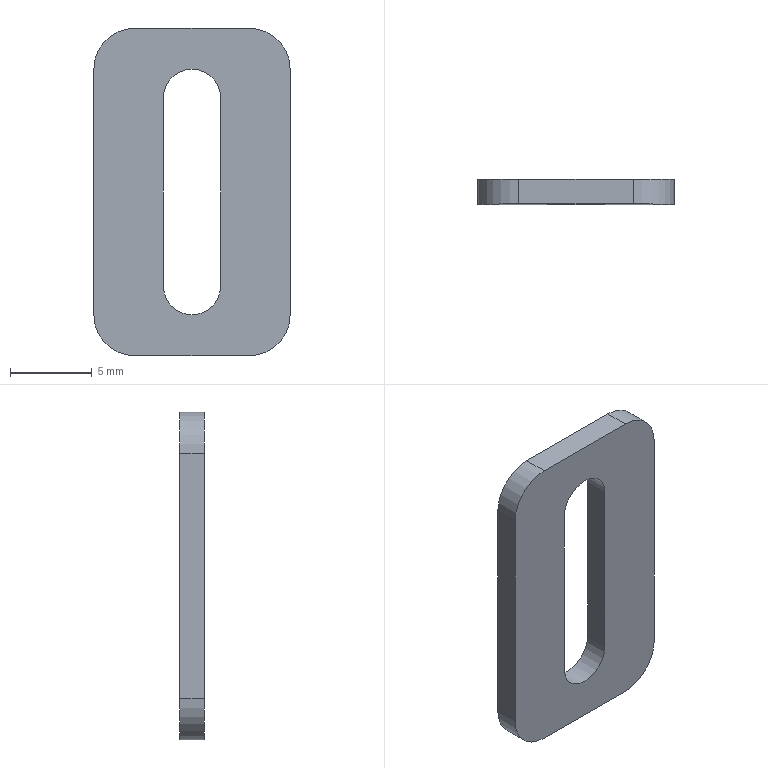Part | STEP file | Glass fixing block 001 | 1 solid | 15 faces | box 12 x 1.5 x 20 mm | volume 277.146 mm3 | plane 8 | cylinder 7 | commonest cylinder face diameters 5 x4 3.5 x3
STEP:
#1=CARTESIAN_POINT('',(0.,0.,0.));
#2=DIRECTION('',(0.,0.,1.));
#3=DIRECTION('',(1.,0.,0.));
#4=AXIS2_PLACEMENT_3D('',#1,#2,#3);
#5=CARTESIAN_POINT('',(1.75,0.,5.75));
#6=VERTEX_POINT('',#5);
#7=CARTESIAN_POINT('',(1.75,1.5,5.75));
#8=VERTEX_POINT('',#7);
#9=CARTESIAN_POINT('',(1.75,0.,5.75));
#10=DIRECTION('',(0.,1.,0.));
#11=VECTOR('',#10,1.);
#12=LINE('',#9,#11);
#13=CARTESIAN_POINT('',(0.,0.,5.75));
#14=DIRECTION('',(0.,1.,0.));
#15=DIRECTION('',(0.,0.,1.));
#16=AXIS2_PLACEMENT_3D('',#13,#14,#15);
#17=CYLINDRICAL_SURFACE('',#16,1.75);
#18=CARTESIAN_POINT('',(1.571,0.));
#19=DIRECTION('',(0.,1.));
#20=VECTOR('',#19,1.);
#21=LINE('',#18,#20);
#22=(GEOMETRIC_REPRESENTATION_CONTEXT(2)PARAMETRIC_REPRESENTATION_CONTEXT()REPRESENTATION_CONTEXT('',''));
#23=DEFINITIONAL_REPRESENTATION('',(#21),#22);
#24=PCURVE('',#17,#23);
#25=CARTESIAN_POINT('',(1.75,0.,5.75));
#26=DIRECTION('',(1.,0.,0.));
#27=DIRECTION('',(0.,0.,-1.));
#28=AXIS2_PLACEMENT_3D('',#25,#26,#27);
#29=PLANE('',#28);
#30=CARTESIAN_POINT('',(0.,0.));
#31=DIRECTION('',(0.,1.));
#32=VECTOR('',#31,1.);
#33=LINE('',#30,#32);
#34=(GEOMETRIC_REPRESENTATION_CONTEXT(2)PARAMETRIC_REPRESENTATION_CONTEXT()REPRESENTATION_CONTEXT('',''));
#35=DEFINITIONAL_REPRESENTATION('',(#33),#34);
#36=PCURVE('',#29,#35);
#37=SURFACE_CURVE('',#12,(#24,#36),.PCURVE_S1.);
#38=EDGE_CURVE('',#6,#8,#37,.T.);
#39=ORIENTED_EDGE('',*,*,#38,.T.);
#40=CARTESIAN_POINT('',(0.,1.5,7.5));
#41=VERTEX_POINT('',#40);
#42=CARTESIAN_POINT('',(0.,1.5,5.75));
#43=DIRECTION('',(0.,1.,0.));
#44=DIRECTION('',(0.,0.,1.));
#45=AXIS2_PLACEMENT_3D('',#42,#43,#44);
#46=CIRCLE('',#45,1.75);
#47=CARTESIAN_POINT('',(0.,1.5));
#48=DIRECTION('',(1.,0.));
#49=VECTOR('',#48,1.);
#50=LINE('',#47,#49);
#51=(GEOMETRIC_REPRESENTATION_CONTEXT(2)PARAMETRIC_REPRESENTATION_CONTEXT()REPRESENTATION_CONTEXT('',''));
#52=DEFINITIONAL_REPRESENTATION('',(#50),#51);
#53=PCURVE('',#17,#52);
#54=CARTESIAN_POINT('',(0.,1.5,0.));
#55=DIRECTION('',(0.,-1.,0.));
#56=DIRECTION('',(0.,0.,-1.));
#57=AXIS2_PLACEMENT_3D('',#54,#55,#56);
#58=PLANE('',#57);
#59=CARTESIAN_POINT('',(-7.5,0.));
#60=CARTESIAN_POINT('',(-7.5,3.031));
#61=CARTESIAN_POINT('',(-4.875,1.516));
#62=CARTESIAN_POINT('',(-2.25,0.));
#63=CARTESIAN_POINT('',(-4.875,-1.516));
#64=CARTESIAN_POINT('',(-7.5,-3.031));
#65=CARTESIAN_POINT('',(-7.5,0.));
#66=(BOUNDED_CURVE()B_SPLINE_CURVE(2,(#59,#60,#61,#62,#63,#64,#65),.UNSPECIFIED.,.T.,.F.)B_SPLINE_CURVE_WITH_KNOTS((1,2,2,2,2,1),(-2.094,0.,2.094,4.189,6.283,8.378),.UNSPECIFIED.)CURVE()GEOMETRIC_REPRESENTATION_ITEM()RATIONAL_B_SPLINE_CURVE((1.,0.5,1.,0.5,1.,0.5,1.))REPRESENTATION_ITEM(''));
#67=(GEOMETRIC_REPRESENTATION_CONTEXT(2)PARAMETRIC_REPRESENTATION_CONTEXT()REPRESENTATION_CONTEXT('',''));
#68=DEFINITIONAL_REPRESENTATION('',(#66),#67);
#69=PCURVE('',#58,#68);
#70=SURFACE_CURVE('',#46,(#53,#69),.PCURVE_S1.);
#71=EDGE_CURVE('',#41,#8,#70,.T.);
#72=ORIENTED_EDGE('',*,*,#71,.F.);
#73=CARTESIAN_POINT('',(0.,0.,7.5));
#74=VERTEX_POINT('',#73);
#75=CARTESIAN_POINT('',(0.,0.,7.5));
#76=DIRECTION('',(0.,1.,0.));
#77=VECTOR('',#76,1.);
#78=LINE('',#75,#77);
#79=CARTESIAN_POINT('',(0.,0.));
#80=DIRECTION('',(0.,1.));
#81=VECTOR('',#80,1.);
#82=LINE('',#79,#81);
#83=(GEOMETRIC_REPRESENTATION_CONTEXT(2)PARAMETRIC_REPRESENTATION_CONTEXT()REPRESENTATION_CONTEXT('',''));
#84=DEFINITIONAL_REPRESENTATION('',(#82),#83);
#85=PCURVE('',#17,#84);
#86=CARTESIAN_POINT('',(0.,0.,5.75));
#87=DIRECTION('',(0.,1.,0.));
#88=DIRECTION('',(0.,0.,1.));
#89=AXIS2_PLACEMENT_3D('',#86,#87,#88);
#90=CYLINDRICAL_SURFACE('',#89,1.75);
#91=CARTESIAN_POINT('',(6.283,0.));
#92=DIRECTION('',(0.,1.));
#93=VECTOR('',#92,1.);
#94=LINE('',#91,#93);
#95=(GEOMETRIC_REPRESENTATION_CONTEXT(2)PARAMETRIC_REPRESENTATION_CONTEXT()REPRESENTATION_CONTEXT('',''));
#96=DEFINITIONAL_REPRESENTATION('',(#94),#95);
#97=PCURVE('',#90,#96);
#98=SURFACE_CURVE('',#78,(#85,#97),.PCURVE_S1.);
#99=EDGE_CURVE('',#74,#41,#98,.T.);
#100=ORIENTED_EDGE('',*,*,#99,.F.);
#101=CARTESIAN_POINT('',(0.,0.,5.75));
#102=DIRECTION('',(0.,1.,0.));
#103=DIRECTION('',(0.,0.,1.));
#104=AXIS2_PLACEMENT_3D('',#101,#102,#103);
#105=CIRCLE('',#104,1.75);
#106=CARTESIAN_POINT('',(0.,0.));
#107=DIRECTION('',(1.,0.));
#108=VECTOR('',#107,1.);
#109=LINE('',#106,#108);
#110=(GEOMETRIC_REPRESENTATION_CONTEXT(2)PARAMETRIC_REPRESENTATION_CONTEXT()REPRESENTATION_CONTEXT('',''));
#111=DEFINITIONAL_REPRESENTATION('',(#109),#110);
#112=PCURVE('',#17,#111);
#113=CARTESIAN_POINT('',(0.,0.,0.));
#114=DIRECTION('',(0.,-1.,0.));
#115=DIRECTION('',(0.,0.,-1.));
#116=AXIS2_PLACEMENT_3D('',#113,#114,#115);
#117=PLANE('',#116);
#118=CARTESIAN_POINT('',(-7.5,0.));
#119=CARTESIAN_POINT('',(-7.5,3.031));
#120=CARTESIAN_POINT('',(-4.875,1.516));
#121=CARTESIAN_POINT('',(-2.25,0.));
#122=CARTESIAN_POINT('',(-4.875,-1.516));
#123=CARTESIAN_POINT('',(-7.5,-3.031));
#124=CARTESIAN_POINT('',(-7.5,0.));
#125=(BOUNDED_CURVE()B_SPLINE_CURVE(2,(#118,#119,#120,#121,#122,#123,#124),.UNSPECIFIED.,.T.,.F.)B_SPLINE_CURVE_WITH_KNOTS((1,2,2,2,2,1),(-2.094,0.,2.094,4.189,6.283,8.378),.UNSPECIFIED.)CURVE()GEOMETRIC_REPRESENTATION_ITEM()RATIONAL_B_SPLINE_CURVE((1.,0.5,1.,0.5,1.,0.5,1.))REPRESENTATION_ITEM(''));
#126=(GEOMETRIC_REPRESENTATION_CONTEXT(2)PARAMETRIC_REPRESENTATION_CONTEXT()REPRESENTATION_CONTEXT('',''));
#127=DEFINITIONAL_REPRESENTATION('',(#125),#126);
#128=PCURVE('',#117,#127);
#129=SURFACE_CURVE('',#105,(#112,#128),.PCURVE_S1.);
#130=EDGE_CURVE('',#74,#6,#129,.T.);
#131=ORIENTED_EDGE('',*,*,#130,.T.);
#132=EDGE_LOOP('',(#39,#72,#100,#131));
#133=FACE_BOUND('',#132,.F.);
#134=ADVANCED_FACE('',(#133),#17,.F.);
#135=CARTESIAN_POINT('',(6.,0.,7.5));
#136=VERTEX_POINT('',#135);
#137=CARTESIAN_POINT('',(6.,0.,-7.5));
#138=VERTEX_POINT('',#137);
#139=CARTESIAN_POINT('',(6.,0.,10.));
#140=DIRECTION('',(0.,0.,-1.));
#141=VECTOR('',#140,1.);
#142=LINE('',#139,#141);
#143=CARTESIAN_POINT('',(6.,1.5,10.));
#144=DIRECTION('',(-1.,0.,0.));
#145=DIRECTION('',(0.,0.,1.));
#146=AXIS2_PLACEMENT_3D('',#143,#144,#145);
#147=PLANE('',#146);
#148=CARTESIAN_POINT('',(0.,-1.5));
#149=DIRECTION('',(-1.,0.));
#150=VECTOR('',#149,1.);
#151=LINE('',#148,#150);
#152=(GEOMETRIC_REPRESENTATION_CONTEXT(2)PARAMETRIC_REPRESENTATION_CONTEXT()REPRESENTATION_CONTEXT('',''));
#153=DEFINITIONAL_REPRESENTATION('',(#151),#152);
#154=PCURVE('',#147,#153);
#155=CARTESIAN_POINT('',(-10.,6.));
#156=DIRECTION('',(1.,0.));
#157=VECTOR('',#156,1.);
#158=LINE('',#155,#157);
#159=(GEOMETRIC_REPRESENTATION_CONTEXT(2)PARAMETRIC_REPRESENTATION_CONTEXT()REPRESENTATION_CONTEXT('',''));
#160=DEFINITIONAL_REPRESENTATION('',(#158),#159);
#161=PCURVE('',#117,#160);
#162=SURFACE_CURVE('',#142,(#154,#161),.PCURVE_S1.);
#163=EDGE_CURVE('',#136,#138,#162,.T.);
#164=ORIENTED_EDGE('',*,*,#163,.T.);
#165=CARTESIAN_POINT('',(6.,1.5,-7.5));
#166=VERTEX_POINT('',#165);
#167=CARTESIAN_POINT('',(6.,1.5,-7.5));
#168=DIRECTION('',(0.,1.,0.));
#169=VECTOR('',#168,1.);
#170=LINE('',#167,#169);
#171=CARTESIAN_POINT('',(-17.5,0.));
#172=DIRECTION('',(0.,1.));
#173=VECTOR('',#172,1.);
#174=LINE('',#171,#173);
#175=(GEOMETRIC_REPRESENTATION_CONTEXT(2)PARAMETRIC_REPRESENTATION_CONTEXT()REPRESENTATION_CONTEXT('',''));
#176=DEFINITIONAL_REPRESENTATION('',(#174),#175);
#177=PCURVE('',#147,#176);
#178=CARTESIAN_POINT('',(3.5,1.5,-7.5));
#179=DIRECTION('',(0.,-1.,0.));
#180=DIRECTION('',(0.,0.,-1.));
#181=AXIS2_PLACEMENT_3D('',#178,#179,#180);
#182=CYLINDRICAL_SURFACE('',#181,2.5);
#183=CARTESIAN_POINT('',(1.571,0.));
#184=DIRECTION('',(0.,-1.));
#185=VECTOR('',#184,1.);
#186=LINE('',#183,#185);
#187=(GEOMETRIC_REPRESENTATION_CONTEXT(2)PARAMETRIC_REPRESENTATION_CONTEXT()REPRESENTATION_CONTEXT('',''));
#188=DEFINITIONAL_REPRESENTATION('',(#186),#187);
#189=PCURVE('',#182,#188);
#190=SURFACE_CURVE('',#170,(#177,#189),.PCURVE_S1.);
#191=EDGE_CURVE('',#138,#166,#190,.T.);
#192=ORIENTED_EDGE('',*,*,#191,.T.);
#193=CARTESIAN_POINT('',(6.,1.5,7.5));
#194=VERTEX_POINT('',#193);
#195=CARTESIAN_POINT('',(6.,1.5,10.));
#196=DIRECTION('',(0.,0.,-1.));
#197=VECTOR('',#196,1.);
#198=LINE('',#195,#197);
#199=CARTESIAN_POINT('',(0.,0.));
#200=DIRECTION('',(-1.,0.));
#201=VECTOR('',#200,1.);
#202=LINE('',#199,#201);
#203=(GEOMETRIC_REPRESENTATION_CONTEXT(2)PARAMETRIC_REPRESENTATION_CONTEXT()REPRESENTATION_CONTEXT('',''));
#204=DEFINITIONAL_REPRESENTATION('',(#202),#203);
#205=PCURVE('',#147,#204);
#206=CARTESIAN_POINT('',(-10.,6.));
#207=DIRECTION('',(1.,0.));
#208=VECTOR('',#207,1.);
#209=LINE('',#206,#208);
#210=(GEOMETRIC_REPRESENTATION_CONTEXT(2)PARAMETRIC_REPRESENTATION_CONTEXT()REPRESENTATION_CONTEXT('',''));
#211=DEFINITIONAL_REPRESENTATION('',(#209),#210);
#212=PCURVE('',#58,#211);
#213=SURFACE_CURVE('',#198,(#205,#212),.PCURVE_S1.);
#214=EDGE_CURVE('',#194,#166,#213,.T.);
#215=ORIENTED_EDGE('',*,*,#214,.F.);
#216=CARTESIAN_POINT('',(6.,1.5,7.5));
#217=DIRECTION('',(0.,-1.,0.));
#218=VECTOR('',#217,1.);
#219=LINE('',#216,#218);
#220=CARTESIAN_POINT('',(-2.5,0.));
#221=DIRECTION('',(0.,-1.));
#222=VECTOR('',#221,1.);
#223=LINE('',#220,#222);
#224=(GEOMETRIC_REPRESENTATION_CONTEXT(2)PARAMETRIC_REPRESENTATION_CONTEXT()REPRESENTATION_CONTEXT('',''));
#225=DEFINITIONAL_REPRESENTATION('',(#223),#224);
#226=PCURVE('',#147,#225);
#227=CARTESIAN_POINT('',(3.5,1.5,7.5));
#228=DIRECTION('',(0.,-1.,0.));
#229=DIRECTION('',(0.,0.,-1.));
#230=AXIS2_PLACEMENT_3D('',#227,#228,#229);
#231=CYLINDRICAL_SURFACE('',#230,2.5);
#232=CARTESIAN_POINT('',(1.571,0.));
#233=DIRECTION('',(0.,1.));
#234=VECTOR('',#233,1.);
#235=LINE('',#232,#234);
#236=(GEOMETRIC_REPRESENTATION_CONTEXT(2)PARAMETRIC_REPRESENTATION_CONTEXT()REPRESENTATION_CONTEXT('',''));
#237=DEFINITIONAL_REPRESENTATION('',(#235),#236);
#238=PCURVE('',#231,#237);
#239=SURFACE_CURVE('',#219,(#226,#238),.PCURVE_S1.);
#240=EDGE_CURVE('',#194,#136,#239,.T.);
#241=ORIENTED_EDGE('',*,*,#240,.T.);
#242=EDGE_LOOP('',(#164,#192,#215,#241));
#243=FACE_BOUND('',#242,.T.);
#244=ADVANCED_FACE('',(#243),#147,.F.);
#245=CARTESIAN_POINT('',(3.5,0.,-10.));
#246=VERTEX_POINT('',#245);
#247=CARTESIAN_POINT('',(-3.5,0.,-10.));
#248=VERTEX_POINT('',#247);
#249=CARTESIAN_POINT('',(-6.,0.,-10.));
#250=DIRECTION('',(-1.,0.,0.));
#251=VECTOR('',#250,1.);
#252=LINE('',#249,#251);
#253=CARTESIAN_POINT('',(-6.,1.5,-10.));
#254=DIRECTION('',(0.,0.,1.));
#255=DIRECTION('',(1.,0.,0.));
#256=AXIS2_PLACEMENT_3D('',#253,#254,#255);
#257=PLANE('',#256);
#258=CARTESIAN_POINT('',(0.,-1.5));
#259=DIRECTION('',(-1.,0.));
#260=VECTOR('',#259,1.);
#261=LINE('',#258,#260);
#262=(GEOMETRIC_REPRESENTATION_CONTEXT(2)PARAMETRIC_REPRESENTATION_CONTEXT()REPRESENTATION_CONTEXT('',''));
#263=DEFINITIONAL_REPRESENTATION('',(#261),#262);
#264=PCURVE('',#257,#263);
#265=CARTESIAN_POINT('',(10.,-6.));
#266=DIRECTION('',(0.,-1.));
#267=VECTOR('',#266,1.);
#268=LINE('',#265,#267);
#269=(GEOMETRIC_REPRESENTATION_CONTEXT(2)PARAMETRIC_REPRESENTATION_CONTEXT()REPRESENTATION_CONTEXT('',''));
#270=DEFINITIONAL_REPRESENTATION('',(#268),#269);
#271=PCURVE('',#117,#270);
#272=SURFACE_CURVE('',#252,(#264,#271),.PCURVE_S1.);
#273=EDGE_CURVE('',#246,#248,#272,.T.);
#274=ORIENTED_EDGE('',*,*,#273,.T.);
#275=CARTESIAN_POINT('',(-3.5,1.5,-10.));
#276=VERTEX_POINT('',#275);
#277=CARTESIAN_POINT('',(-3.5,1.5,-10.));
#278=DIRECTION('',(0.,1.,0.));
#279=VECTOR('',#278,1.);
#280=LINE('',#277,#279);
#281=CARTESIAN_POINT('',(2.5,0.));
#282=DIRECTION('',(0.,1.));
#283=VECTOR('',#282,1.);
#284=LINE('',#281,#283);
#285=(GEOMETRIC_REPRESENTATION_CONTEXT(2)PARAMETRIC_REPRESENTATION_CONTEXT()REPRESENTATION_CONTEXT('',''));
#286=DEFINITIONAL_REPRESENTATION('',(#284),#285);
#287=PCURVE('',#257,#286);
#288=CARTESIAN_POINT('',(-3.5,1.5,-7.5));
#289=DIRECTION('',(0.,-1.,0.));
#290=DIRECTION('',(0.,0.,-1.));
#291=AXIS2_PLACEMENT_3D('',#288,#289,#290);
#292=CYLINDRICAL_SURFACE('',#291,2.5);
#293=CARTESIAN_POINT('',(6.283,0.));
#294=DIRECTION('',(0.,-1.));
#295=VECTOR('',#294,1.);
#296=LINE('',#293,#295);
#297=(GEOMETRIC_REPRESENTATION_CONTEXT(2)PARAMETRIC_REPRESENTATION_CONTEXT()REPRESENTATION_CONTEXT('',''));
#298=DEFINITIONAL_REPRESENTATION('',(#296),#297);
#299=PCURVE('',#292,#298);
#300=SURFACE_CURVE('',#280,(#287,#299),.PCURVE_S1.);
#301=EDGE_CURVE('',#248,#276,#300,.T.);
#302=ORIENTED_EDGE('',*,*,#301,.T.);
#303=CARTESIAN_POINT('',(3.5,1.5,-10.));
#304=VERTEX_POINT('',#303);
#305=CARTESIAN_POINT('',(-6.,1.5,-10.));
#306=DIRECTION('',(-1.,0.,0.));
#307=VECTOR('',#306,1.);
#308=LINE('',#305,#307);
#309=CARTESIAN_POINT('',(0.,0.));
#310=DIRECTION('',(-1.,0.));
#311=VECTOR('',#310,1.);
#312=LINE('',#309,#311);
#313=(GEOMETRIC_REPRESENTATION_CONTEXT(2)PARAMETRIC_REPRESENTATION_CONTEXT()REPRESENTATION_CONTEXT('',''));
#314=DEFINITIONAL_REPRESENTATION('',(#312),#313);
#315=PCURVE('',#257,#314);
#316=CARTESIAN_POINT('',(10.,-6.));
#317=DIRECTION('',(0.,-1.));
#318=VECTOR('',#317,1.);
#319=LINE('',#316,#318);
#320=(GEOMETRIC_REPRESENTATION_CONTEXT(2)PARAMETRIC_REPRESENTATION_CONTEXT()REPRESENTATION_CONTEXT('',''));
#321=DEFINITIONAL_REPRESENTATION('',(#319),#320);
#322=PCURVE('',#58,#321);
#323=SURFACE_CURVE('',#308,(#315,#322),.PCURVE_S1.);
#324=EDGE_CURVE('',#304,#276,#323,.T.);
#325=ORIENTED_EDGE('',*,*,#324,.F.);
#326=CARTESIAN_POINT('',(3.5,1.5,-10.));
#327=DIRECTION('',(0.,-1.,0.));
#328=VECTOR('',#327,1.);
#329=LINE('',#326,#328);
#330=CARTESIAN_POINT('',(9.5,0.));
#331=DIRECTION('',(0.,-1.));
#332=VECTOR('',#331,1.);
#333=LINE('',#330,#332);
#334=(GEOMETRIC_REPRESENTATION_CONTEXT(2)PARAMETRIC_REPRESENTATION_CONTEXT()REPRESENTATION_CONTEXT('',''));
#335=DEFINITIONAL_REPRESENTATION('',(#333),#334);
#336=PCURVE('',#257,#335);
#337=CARTESIAN_POINT('',(0.,0.));
#338=DIRECTION('',(0.,1.));
#339=VECTOR('',#338,1.);
#340=LINE('',#337,#339);
#341=(GEOMETRIC_REPRESENTATION_CONTEXT(2)PARAMETRIC_REPRESENTATION_CONTEXT()REPRESENTATION_CONTEXT('',''));
#342=DEFINITIONAL_REPRESENTATION('',(#340),#341);
#343=PCURVE('',#182,#342);
#344=SURFACE_CURVE('',#329,(#336,#343),.PCURVE_S1.);
#345=EDGE_CURVE('',#304,#246,#344,.T.);
#346=ORIENTED_EDGE('',*,*,#345,.T.);
#347=EDGE_LOOP('',(#274,#302,#325,#346));
#348=FACE_BOUND('',#347,.T.);
#349=ADVANCED_FACE('',(#348),#257,.F.);
#350=CARTESIAN_POINT('',(-6.,0.,-7.5));
#351=VERTEX_POINT('',#350);
#352=CARTESIAN_POINT('',(-6.,0.,7.5));
#353=VERTEX_POINT('',#352);
#354=CARTESIAN_POINT('',(-6.,0.,10.));
#355=DIRECTION('',(0.,0.,1.));
#356=VECTOR('',#355,1.);
#357=LINE('',#354,#356);
#358=CARTESIAN_POINT('',(-6.,1.5,10.));
#359=DIRECTION('',(1.,0.,0.));
#360=DIRECTION('',(0.,0.,-1.));
#361=AXIS2_PLACEMENT_3D('',#358,#359,#360);
#362=PLANE('',#361);
#363=CARTESIAN_POINT('',(0.,-1.5));
#364=DIRECTION('',(-1.,0.));
#365=VECTOR('',#364,1.);
#366=LINE('',#363,#365);
#367=(GEOMETRIC_REPRESENTATION_CONTEXT(2)PARAMETRIC_REPRESENTATION_CONTEXT()REPRESENTATION_CONTEXT('',''));
#368=DEFINITIONAL_REPRESENTATION('',(#366),#367);
#369=PCURVE('',#362,#368);
#370=CARTESIAN_POINT('',(-10.,-6.));
#371=DIRECTION('',(-1.,0.));
#372=VECTOR('',#371,1.);
#373=LINE('',#370,#372);
#374=(GEOMETRIC_REPRESENTATION_CONTEXT(2)PARAMETRIC_REPRESENTATION_CONTEXT()REPRESENTATION_CONTEXT('',''));
#375=DEFINITIONAL_REPRESENTATION('',(#373),#374);
#376=PCURVE('',#117,#375);
#377=SURFACE_CURVE('',#357,(#369,#376),.PCURVE_S1.);
#378=EDGE_CURVE('',#351,#353,#377,.T.);
#379=ORIENTED_EDGE('',*,*,#378,.T.);
#380=CARTESIAN_POINT('',(-6.,1.5,7.5));
#381=VERTEX_POINT('',#380);
#382=CARTESIAN_POINT('',(-6.,1.5,7.5));
#383=DIRECTION('',(0.,1.,0.));
#384=VECTOR('',#383,1.);
#385=LINE('',#382,#384);
#386=CARTESIAN_POINT('',(2.5,0.));
#387=DIRECTION('',(0.,1.));
#388=VECTOR('',#387,1.);
#389=LINE('',#386,#388);
#390=(GEOMETRIC_REPRESENTATION_CONTEXT(2)PARAMETRIC_REPRESENTATION_CONTEXT()REPRESENTATION_CONTEXT('',''));
#391=DEFINITIONAL_REPRESENTATION('',(#389),#390);
#392=PCURVE('',#362,#391);
#393=CARTESIAN_POINT('',(-3.5,1.5,7.5));
#394=DIRECTION('',(0.,-1.,0.));
#395=DIRECTION('',(0.,0.,-1.));
#396=AXIS2_PLACEMENT_3D('',#393,#394,#395);
#397=CYLINDRICAL_SURFACE('',#396,2.5);
#398=CARTESIAN_POINT('',(4.712,0.));
#399=DIRECTION('',(0.,-1.));
#400=VECTOR('',#399,1.);
#401=LINE('',#398,#400);
#402=(GEOMETRIC_REPRESENTATION_CONTEXT(2)PARAMETRIC_REPRESENTATION_CONTEXT()REPRESENTATION_CONTEXT('',''));
#403=DEFINITIONAL_REPRESENTATION('',(#401),#402);
#404=PCURVE('',#397,#403);
#405=SURFACE_CURVE('',#385,(#392,#404),.PCURVE_S1.);
#406=EDGE_CURVE('',#353,#381,#405,.T.);
#407=ORIENTED_EDGE('',*,*,#406,.T.);
#408=CARTESIAN_POINT('',(-6.,1.5,-7.5));
#409=VERTEX_POINT('',#408);
#410=CARTESIAN_POINT('',(-6.,1.5,10.));
#411=DIRECTION('',(0.,0.,1.));
#412=VECTOR('',#411,1.);
#413=LINE('',#410,#412);
#414=CARTESIAN_POINT('',(0.,0.));
#415=DIRECTION('',(-1.,0.));
#416=VECTOR('',#415,1.);
#417=LINE('',#414,#416);
#418=(GEOMETRIC_REPRESENTATION_CONTEXT(2)PARAMETRIC_REPRESENTATION_CONTEXT()REPRESENTATION_CONTEXT('',''));
#419=DEFINITIONAL_REPRESENTATION('',(#417),#418);
#420=PCURVE('',#362,#419);
#421=CARTESIAN_POINT('',(-10.,-6.));
#422=DIRECTION('',(-1.,0.));
#423=VECTOR('',#422,1.);
#424=LINE('',#421,#423);
#425=(GEOMETRIC_REPRESENTATION_CONTEXT(2)PARAMETRIC_REPRESENTATION_CONTEXT()REPRESENTATION_CONTEXT('',''));
#426=DEFINITIONAL_REPRESENTATION('',(#424),#425);
#427=PCURVE('',#58,#426);
#428=SURFACE_CURVE('',#413,(#420,#427),.PCURVE_S1.);
#429=EDGE_CURVE('',#409,#381,#428,.T.);
#430=ORIENTED_EDGE('',*,*,#429,.F.);
#431=CARTESIAN_POINT('',(-6.,1.5,-7.5));
#432=DIRECTION('',(0.,-1.,0.));
#433=VECTOR('',#432,1.);
#434=LINE('',#431,#433);
#435=CARTESIAN_POINT('',(17.5,0.));
#436=DIRECTION('',(0.,-1.));
#437=VECTOR('',#436,1.);
#438=LINE('',#435,#437);
#439=(GEOMETRIC_REPRESENTATION_CONTEXT(2)PARAMETRIC_REPRESENTATION_CONTEXT()REPRESENTATION_CONTEXT('',''));
#440=DEFINITIONAL_REPRESENTATION('',(#438),#439);
#441=PCURVE('',#362,#440);
#442=CARTESIAN_POINT('',(4.712,0.));
#443=DIRECTION('',(0.,1.));
#444=VECTOR('',#443,1.);
#445=LINE('',#442,#444);
#446=(GEOMETRIC_REPRESENTATION_CONTEXT(2)PARAMETRIC_REPRESENTATION_CONTEXT()REPRESENTATION_CONTEXT('',''));
#447=DEFINITIONAL_REPRESENTATION('',(#445),#446);
#448=PCURVE('',#292,#447);
#449=SURFACE_CURVE('',#434,(#441,#448),.PCURVE_S1.);
#450=EDGE_CURVE('',#409,#351,#449,.T.);
#451=ORIENTED_EDGE('',*,*,#450,.T.);
#452=EDGE_LOOP('',(#379,#407,#430,#451));
#453=FACE_BOUND('',#452,.T.);
#454=ADVANCED_FACE('',(#453),#362,.F.);
#455=CARTESIAN_POINT('',(-3.5,1.5,10.));
#456=VERTEX_POINT('',#455);
#457=CARTESIAN_POINT('',(3.5,1.5,10.));
#458=VERTEX_POINT('',#457);
#459=CARTESIAN_POINT('',(-6.,1.5,10.));
#460=DIRECTION('',(1.,0.,0.));
#461=VECTOR('',#460,1.);
#462=LINE('',#459,#461);
#463=CARTESIAN_POINT('',(-6.,1.5,10.));
#464=DIRECTION('',(0.,0.,-1.));
#465=DIRECTION('',(-1.,0.,0.));
#466=AXIS2_PLACEMENT_3D('',#463,#464,#465);
#467=PLANE('',#466);
#468=CARTESIAN_POINT('',(0.,0.));
#469=DIRECTION('',(-1.,0.));
#470=VECTOR('',#469,1.);
#471=LINE('',#468,#470);
#472=(GEOMETRIC_REPRESENTATION_CONTEXT(2)PARAMETRIC_REPRESENTATION_CONTEXT()REPRESENTATION_CONTEXT('',''));
#473=DEFINITIONAL_REPRESENTATION('',(#471),#472);
#474=PCURVE('',#467,#473);
#475=CARTESIAN_POINT('',(-10.,-6.));
#476=DIRECTION('',(0.,1.));
#477=VECTOR('',#476,1.);
#478=LINE('',#475,#477);
#479=(GEOMETRIC_REPRESENTATION_CONTEXT(2)PARAMETRIC_REPRESENTATION_CONTEXT()REPRESENTATION_CONTEXT('',''));
#480=DEFINITIONAL_REPRESENTATION('',(#478),#479);
#481=PCURVE('',#58,#480);
#482=SURFACE_CURVE('',#462,(#474,#481),.PCURVE_S1.);
#483=EDGE_CURVE('',#456,#458,#482,.T.);
#484=ORIENTED_EDGE('',*,*,#483,.F.);
#485=CARTESIAN_POINT('',(-3.5,0.,10.));
#486=VERTEX_POINT('',#485);
#487=CARTESIAN_POINT('',(-3.5,1.5,10.));
#488=DIRECTION('',(0.,-1.,0.));
#489=VECTOR('',#488,1.);
#490=LINE('',#487,#489);
#491=CARTESIAN_POINT('',(-2.5,0.));
#492=DIRECTION('',(0.,-1.));
#493=VECTOR('',#492,1.);
#494=LINE('',#491,#493);
#495=(GEOMETRIC_REPRESENTATION_CONTEXT(2)PARAMETRIC_REPRESENTATION_CONTEXT()REPRESENTATION_CONTEXT('',''));
#496=DEFINITIONAL_REPRESENTATION('',(#494),#495);
#497=PCURVE('',#467,#496);
#498=CARTESIAN_POINT('',(3.142,0.));
#499=DIRECTION('',(0.,1.));
#500=VECTOR('',#499,1.);
#501=LINE('',#498,#500);
#502=(GEOMETRIC_REPRESENTATION_CONTEXT(2)PARAMETRIC_REPRESENTATION_CONTEXT()REPRESENTATION_CONTEXT('',''));
#503=DEFINITIONAL_REPRESENTATION('',(#501),#502);
#504=PCURVE('',#397,#503);
#505=SURFACE_CURVE('',#490,(#497,#504),.PCURVE_S1.);
#506=EDGE_CURVE('',#456,#486,#505,.T.);
#507=ORIENTED_EDGE('',*,*,#506,.T.);
#508=CARTESIAN_POINT('',(3.5,0.,10.));
#509=VERTEX_POINT('',#508);
#510=CARTESIAN_POINT('',(-6.,0.,10.));
#511=DIRECTION('',(1.,0.,0.));
#512=VECTOR('',#511,1.);
#513=LINE('',#510,#512);
#514=CARTESIAN_POINT('',(0.,-1.5));
#515=DIRECTION('',(-1.,0.));
#516=VECTOR('',#515,1.);
#517=LINE('',#514,#516);
#518=(GEOMETRIC_REPRESENTATION_CONTEXT(2)PARAMETRIC_REPRESENTATION_CONTEXT()REPRESENTATION_CONTEXT('',''));
#519=DEFINITIONAL_REPRESENTATION('',(#517),#518);
#520=PCURVE('',#467,#519);
#521=CARTESIAN_POINT('',(-10.,-6.));
#522=DIRECTION('',(0.,1.));
#523=VECTOR('',#522,1.);
#524=LINE('',#521,#523);
#525=(GEOMETRIC_REPRESENTATION_CONTEXT(2)PARAMETRIC_REPRESENTATION_CONTEXT()REPRESENTATION_CONTEXT('',''));
#526=DEFINITIONAL_REPRESENTATION('',(#524),#525);
#527=PCURVE('',#117,#526);
#528=SURFACE_CURVE('',#513,(#520,#527),.PCURVE_S1.);
#529=EDGE_CURVE('',#486,#509,#528,.T.);
#530=ORIENTED_EDGE('',*,*,#529,.T.);
#531=CARTESIAN_POINT('',(3.5,1.5,10.));
#532=DIRECTION('',(0.,1.,0.));
#533=VECTOR('',#532,1.);
#534=LINE('',#531,#533);
#535=CARTESIAN_POINT('',(-9.5,0.));
#536=DIRECTION('',(0.,1.));
#537=VECTOR('',#536,1.);
#538=LINE('',#535,#537);
#539=(GEOMETRIC_REPRESENTATION_CONTEXT(2)PARAMETRIC_REPRESENTATION_CONTEXT()REPRESENTATION_CONTEXT('',''));
#540=DEFINITIONAL_REPRESENTATION('',(#538),#539);
#541=PCURVE('',#467,#540);
#542=CARTESIAN_POINT('',(3.142,0.));
#543=DIRECTION('',(0.,-1.));
#544=VECTOR('',#543,1.);
#545=LINE('',#542,#544);
#546=(GEOMETRIC_REPRESENTATION_CONTEXT(2)PARAMETRIC_REPRESENTATION_CONTEXT()REPRESENTATION_CONTEXT('',''));
#547=DEFINITIONAL_REPRESENTATION('',(#545),#546);
#548=PCURVE('',#231,#547);
#549=SURFACE_CURVE('',#534,(#541,#548),.PCURVE_S1.);
#550=EDGE_CURVE('',#509,#458,#549,.T.);
#551=ORIENTED_EDGE('',*,*,#550,.T.);
#552=EDGE_LOOP('',(#484,#507,#530,#551));
#553=FACE_BOUND('',#552,.T.);
#554=ADVANCED_FACE('',(#553),#467,.F.);
#555=CARTESIAN_POINT('',(1.75,1.5,-5.75));
#556=VERTEX_POINT('',#555);
#557=CARTESIAN_POINT('',(1.75,1.5,5.75));
#558=DIRECTION('',(0.,0.,-1.));
#559=VECTOR('',#558,1.);
#560=LINE('',#557,#559);
#561=CARTESIAN_POINT('',(-5.75,1.75));
#562=DIRECTION('',(1.,0.));
#563=VECTOR('',#562,1.);
#564=LINE('',#561,#563);
#565=(GEOMETRIC_REPRESENTATION_CONTEXT(2)PARAMETRIC_REPRESENTATION_CONTEXT()REPRESENTATION_CONTEXT('',''));
#566=DEFINITIONAL_REPRESENTATION('',(#564),#565);
#567=PCURVE('',#58,#566);
#568=CARTESIAN_POINT('',(0.,1.5));
#569=DIRECTION('',(1.,0.));
#570=VECTOR('',#569,1.);
#571=LINE('',#568,#570);
#572=(GEOMETRIC_REPRESENTATION_CONTEXT(2)PARAMETRIC_REPRESENTATION_CONTEXT()REPRESENTATION_CONTEXT('',''));
#573=DEFINITIONAL_REPRESENTATION('',(#571),#572);
#574=PCURVE('',#29,#573);
#575=SURFACE_CURVE('',#560,(#567,#574),.PCURVE_S1.);
#576=EDGE_CURVE('',#8,#556,#575,.T.);
#577=ORIENTED_EDGE('',*,*,#576,.F.);
#578=ORIENTED_EDGE('',*,*,#71,.F.);
#579=CARTESIAN_POINT('',(-1.75,1.5,5.75));
#580=VERTEX_POINT('',#579);
#581=CARTESIAN_POINT('',(0.,1.5,5.75));
#582=DIRECTION('',(0.,1.,0.));
#583=DIRECTION('',(0.,0.,1.));
#584=AXIS2_PLACEMENT_3D('',#581,#582,#583);
#585=CIRCLE('',#584,1.75);
#586=CARTESIAN_POINT('',(-7.5,0.));
#587=CARTESIAN_POINT('',(-7.5,3.031));
#588=CARTESIAN_POINT('',(-4.875,1.516));
#589=CARTESIAN_POINT('',(-2.25,0.));
#590=CARTESIAN_POINT('',(-4.875,-1.516));
#591=CARTESIAN_POINT('',(-7.5,-3.031));
#592=CARTESIAN_POINT('',(-7.5,0.));
#593=(BOUNDED_CURVE()B_SPLINE_CURVE(2,(#586,#587,#588,#589,#590,#591,#592),.UNSPECIFIED.,.T.,.F.)B_SPLINE_CURVE_WITH_KNOTS((1,2,2,2,2,1),(-2.094,0.,2.094,4.189,6.283,8.378),.UNSPECIFIED.)CURVE()GEOMETRIC_REPRESENTATION_ITEM()RATIONAL_B_SPLINE_CURVE((1.,0.5,1.,0.5,1.,0.5,1.))REPRESENTATION_ITEM(''));
#594=(GEOMETRIC_REPRESENTATION_CONTEXT(2)PARAMETRIC_REPRESENTATION_CONTEXT()REPRESENTATION_CONTEXT('',''));
#595=DEFINITIONAL_REPRESENTATION('',(#593),#594);
#596=PCURVE('',#58,#595);
#597=CARTESIAN_POINT('',(0.,1.5));
#598=DIRECTION('',(1.,0.));
#599=VECTOR('',#598,1.);
#600=LINE('',#597,#599);
#601=(GEOMETRIC_REPRESENTATION_CONTEXT(2)PARAMETRIC_REPRESENTATION_CONTEXT()REPRESENTATION_CONTEXT('',''));
#602=DEFINITIONAL_REPRESENTATION('',(#600),#601);
#603=PCURVE('',#90,#602);
#604=SURFACE_CURVE('',#585,(#596,#603),.PCURVE_S1.);
#605=EDGE_CURVE('',#580,#41,#604,.T.);
#606=ORIENTED_EDGE('',*,*,#605,.F.);
#607=CARTESIAN_POINT('',(-1.75,1.5,-5.75));
#608=VERTEX_POINT('',#607);
#609=CARTESIAN_POINT('',(-1.75,1.5,5.75));
#610=DIRECTION('',(0.,0.,1.));
#611=VECTOR('',#610,1.);
#612=LINE('',#609,#611);
#613=CARTESIAN_POINT('',(-5.75,-1.75));
#614=DIRECTION('',(-1.,0.));
#615=VECTOR('',#614,1.);
#616=LINE('',#613,#615);
#617=(GEOMETRIC_REPRESENTATION_CONTEXT(2)PARAMETRIC_REPRESENTATION_CONTEXT()REPRESENTATION_CONTEXT('',''));
#618=DEFINITIONAL_REPRESENTATION('',(#616),#617);
#619=PCURVE('',#58,#618);
#620=CARTESIAN_POINT('',(-1.75,0.,5.75));
#621=DIRECTION('',(-1.,0.,0.));
#622=DIRECTION('',(0.,0.,1.));
#623=AXIS2_PLACEMENT_3D('',#620,#621,#622);
#624=PLANE('',#623);
#625=CARTESIAN_POINT('',(0.,1.5));
#626=DIRECTION('',(1.,0.));
#627=VECTOR('',#626,1.);
#628=LINE('',#625,#627);
#629=(GEOMETRIC_REPRESENTATION_CONTEXT(2)PARAMETRIC_REPRESENTATION_CONTEXT()REPRESENTATION_CONTEXT('',''));
#630=DEFINITIONAL_REPRESENTATION('',(#628),#629);
#631=PCURVE('',#624,#630);
#632=SURFACE_CURVE('',#612,(#619,#631),.PCURVE_S1.);
#633=EDGE_CURVE('',#608,#580,#632,.T.);
#634=ORIENTED_EDGE('',*,*,#633,.F.);
#635=CARTESIAN_POINT('',(0.,1.5,-5.75));
#636=DIRECTION('',(0.,1.,0.));
#637=DIRECTION('',(0.,0.,1.));
#638=AXIS2_PLACEMENT_3D('',#635,#636,#637);
#639=CIRCLE('',#638,1.75);
#640=CARTESIAN_POINT('',(4.,0.));
#641=CARTESIAN_POINT('',(4.,3.031));
#642=CARTESIAN_POINT('',(6.625,1.516));
#643=CARTESIAN_POINT('',(9.25,0.));
#644=CARTESIAN_POINT('',(6.625,-1.516));
#645=CARTESIAN_POINT('',(4.,-3.031));
#646=CARTESIAN_POINT('',(4.,0.));
#647=(BOUNDED_CURVE()B_SPLINE_CURVE(2,(#640,#641,#642,#643,#644,#645,#646),.UNSPECIFIED.,.T.,.F.)B_SPLINE_CURVE_WITH_KNOTS((1,2,2,2,2,1),(-2.094,0.,2.094,4.189,6.283,8.378),.UNSPECIFIED.)CURVE()GEOMETRIC_REPRESENTATION_ITEM()RATIONAL_B_SPLINE_CURVE((1.,0.5,1.,0.5,1.,0.5,1.))REPRESENTATION_ITEM(''));
#648=(GEOMETRIC_REPRESENTATION_CONTEXT(2)PARAMETRIC_REPRESENTATION_CONTEXT()REPRESENTATION_CONTEXT('',''));
#649=DEFINITIONAL_REPRESENTATION('',(#647),#648);
#650=PCURVE('',#58,#649);
#651=CARTESIAN_POINT('',(0.,0.,-5.75));
#652=DIRECTION('',(0.,1.,0.));
#653=DIRECTION('',(0.,0.,1.));
#654=AXIS2_PLACEMENT_3D('',#651,#652,#653);
#655=CYLINDRICAL_SURFACE('',#654,1.75);
#656=CARTESIAN_POINT('',(0.,1.5));
#657=DIRECTION('',(1.,0.));
#658=VECTOR('',#657,1.);
#659=LINE('',#656,#658);
#660=(GEOMETRIC_REPRESENTATION_CONTEXT(2)PARAMETRIC_REPRESENTATION_CONTEXT()REPRESENTATION_CONTEXT('',''));
#661=DEFINITIONAL_REPRESENTATION('',(#659),#660);
#662=PCURVE('',#655,#661);
#663=SURFACE_CURVE('',#639,(#650,#662),.PCURVE_S1.);
#664=EDGE_CURVE('',#556,#608,#663,.T.);
#665=ORIENTED_EDGE('',*,*,#664,.F.);
#666=EDGE_LOOP('',(#577,#578,#606,#634,#665));
#667=FACE_BOUND('',#666,.T.);
#668=ORIENTED_EDGE('',*,*,#429,.T.);
#669=CARTESIAN_POINT('',(-3.5,1.5,7.5));
#670=DIRECTION('',(0.,1.,0.));
#671=DIRECTION('',(0.,0.,-1.));
#672=AXIS2_PLACEMENT_3D('',#669,#670,#671);
#673=CIRCLE('',#672,2.5);
#674=CARTESIAN_POINT('',(-5.,-3.5));
#675=CARTESIAN_POINT('',(-5.,-7.83));
#676=CARTESIAN_POINT('',(-8.75,-5.665));
#677=CARTESIAN_POINT('',(-12.5,-3.5));
#678=CARTESIAN_POINT('',(-8.75,-1.335));
#679=CARTESIAN_POINT('',(-5.,0.8301));
#680=CARTESIAN_POINT('',(-5.,-3.5));
#681=(BOUNDED_CURVE()B_SPLINE_CURVE(2,(#674,#675,#676,#677,#678,#679,#680),.UNSPECIFIED.,.T.,.F.)B_SPLINE_CURVE_WITH_KNOTS((1,2,2,2,2,1),(-2.094,0.,2.094,4.189,6.283,8.378),.UNSPECIFIED.)CURVE()GEOMETRIC_REPRESENTATION_ITEM()RATIONAL_B_SPLINE_CURVE((1.,0.5,1.,0.5,1.,0.5,1.))REPRESENTATION_ITEM(''));
#682=(GEOMETRIC_REPRESENTATION_CONTEXT(2)PARAMETRIC_REPRESENTATION_CONTEXT()REPRESENTATION_CONTEXT('',''));
#683=DEFINITIONAL_REPRESENTATION('',(#681),#682);
#684=PCURVE('',#58,#683);
#685=CARTESIAN_POINT('',(6.283,0.));
#686=DIRECTION('',(-1.,0.));
#687=VECTOR('',#686,1.);
#688=LINE('',#685,#687);
#689=(GEOMETRIC_REPRESENTATION_CONTEXT(2)PARAMETRIC_REPRESENTATION_CONTEXT()REPRESENTATION_CONTEXT('',''));
#690=DEFINITIONAL_REPRESENTATION('',(#688),#689);
#691=PCURVE('',#397,#690);
#692=SURFACE_CURVE('',#673,(#684,#691),.PCURVE_S1.);
#693=EDGE_CURVE('',#381,#456,#692,.T.);
#694=ORIENTED_EDGE('',*,*,#693,.T.);
#695=ORIENTED_EDGE('',*,*,#483,.T.);
#696=CARTESIAN_POINT('',(3.5,1.5,7.5));
#697=DIRECTION('',(0.,1.,0.));
#698=DIRECTION('',(0.,0.,-1.));
#699=AXIS2_PLACEMENT_3D('',#696,#697,#698);
#700=CIRCLE('',#699,2.5);
#701=CARTESIAN_POINT('',(-5.,3.5));
#702=CARTESIAN_POINT('',(-5.,-0.8301));
#703=CARTESIAN_POINT('',(-8.75,1.335));
#704=CARTESIAN_POINT('',(-12.5,3.5));
#705=CARTESIAN_POINT('',(-8.75,5.665));
#706=CARTESIAN_POINT('',(-5.,7.83));
#707=CARTESIAN_POINT('',(-5.,3.5));
#708=(BOUNDED_CURVE()B_SPLINE_CURVE(2,(#701,#702,#703,#704,#705,#706,#707),.UNSPECIFIED.,.T.,.F.)B_SPLINE_CURVE_WITH_KNOTS((1,2,2,2,2,1),(-2.094,0.,2.094,4.189,6.283,8.378),.UNSPECIFIED.)CURVE()GEOMETRIC_REPRESENTATION_ITEM()RATIONAL_B_SPLINE_CURVE((1.,0.5,1.,0.5,1.,0.5,1.))REPRESENTATION_ITEM(''));
#709=(GEOMETRIC_REPRESENTATION_CONTEXT(2)PARAMETRIC_REPRESENTATION_CONTEXT()REPRESENTATION_CONTEXT('',''));
#710=DEFINITIONAL_REPRESENTATION('',(#708),#709);
#711=PCURVE('',#58,#710);
#712=CARTESIAN_POINT('',(6.283,0.));
#713=DIRECTION('',(-1.,0.));
#714=VECTOR('',#713,1.);
#715=LINE('',#712,#714);
#716=(GEOMETRIC_REPRESENTATION_CONTEXT(2)PARAMETRIC_REPRESENTATION_CONTEXT()REPRESENTATION_CONTEXT('',''));
#717=DEFINITIONAL_REPRESENTATION('',(#715),#716);
#718=PCURVE('',#231,#717);
#719=SURFACE_CURVE('',#700,(#711,#718),.PCURVE_S1.);
#720=EDGE_CURVE('',#458,#194,#719,.T.);
#721=ORIENTED_EDGE('',*,*,#720,.T.);
#722=ORIENTED_EDGE('',*,*,#214,.T.);
#723=CARTESIAN_POINT('',(3.5,1.5,-7.5));
#724=DIRECTION('',(0.,1.,0.));
#725=DIRECTION('',(0.,0.,-1.));
#726=AXIS2_PLACEMENT_3D('',#723,#724,#725);
#727=CIRCLE('',#726,2.5);
#728=CARTESIAN_POINT('',(10.,3.5));
#729=CARTESIAN_POINT('',(10.,-0.8301));
#730=CARTESIAN_POINT('',(6.25,1.335));
#731=CARTESIAN_POINT('',(2.5,3.5));
#732=CARTESIAN_POINT('',(6.25,5.665));
#733=CARTESIAN_POINT('',(10.,7.83));
#734=CARTESIAN_POINT('',(10.,3.5));
#735=(BOUNDED_CURVE()B_SPLINE_CURVE(2,(#728,#729,#730,#731,#732,#733,#734),.UNSPECIFIED.,.T.,.F.)B_SPLINE_CURVE_WITH_KNOTS((1,2,2,2,2,1),(-2.094,0.,2.094,4.189,6.283,8.378),.UNSPECIFIED.)CURVE()GEOMETRIC_REPRESENTATION_ITEM()RATIONAL_B_SPLINE_CURVE((1.,0.5,1.,0.5,1.,0.5,1.))REPRESENTATION_ITEM(''));
#736=(GEOMETRIC_REPRESENTATION_CONTEXT(2)PARAMETRIC_REPRESENTATION_CONTEXT()REPRESENTATION_CONTEXT('',''));
#737=DEFINITIONAL_REPRESENTATION('',(#735),#736);
#738=PCURVE('',#58,#737);
#739=CARTESIAN_POINT('',(6.283,0.));
#740=DIRECTION('',(-1.,0.));
#741=VECTOR('',#740,1.);
#742=LINE('',#739,#741);
#743=(GEOMETRIC_REPRESENTATION_CONTEXT(2)PARAMETRIC_REPRESENTATION_CONTEXT()REPRESENTATION_CONTEXT('',''));
#744=DEFINITIONAL_REPRESENTATION('',(#742),#743);
#745=PCURVE('',#182,#744);
#746=SURFACE_CURVE('',#727,(#738,#745),.PCURVE_S1.);
#747=EDGE_CURVE('',#166,#304,#746,.T.);
#748=ORIENTED_EDGE('',*,*,#747,.T.);
#749=ORIENTED_EDGE('',*,*,#324,.T.);
#750=CARTESIAN_POINT('',(-3.5,1.5,-7.5));
#751=DIRECTION('',(0.,1.,0.));
#752=DIRECTION('',(0.,0.,-1.));
#753=AXIS2_PLACEMENT_3D('',#750,#751,#752);
#754=CIRCLE('',#753,2.5);
#755=CARTESIAN_POINT('',(10.,-3.5));
#756=CARTESIAN_POINT('',(10.,-7.83));
#757=CARTESIAN_POINT('',(6.25,-5.665));
#758=CARTESIAN_POINT('',(2.5,-3.5));
#759=CARTESIAN_POINT('',(6.25,-1.335));
#760=CARTESIAN_POINT('',(10.,0.8301));
#761=CARTESIAN_POINT('',(10.,-3.5));
#762=(BOUNDED_CURVE()B_SPLINE_CURVE(2,(#755,#756,#757,#758,#759,#760,#761),.UNSPECIFIED.,.T.,.F.)B_SPLINE_CURVE_WITH_KNOTS((1,2,2,2,2,1),(-2.094,0.,2.094,4.189,6.283,8.378),.UNSPECIFIED.)CURVE()GEOMETRIC_REPRESENTATION_ITEM()RATIONAL_B_SPLINE_CURVE((1.,0.5,1.,0.5,1.,0.5,1.))REPRESENTATION_ITEM(''));
#763=(GEOMETRIC_REPRESENTATION_CONTEXT(2)PARAMETRIC_REPRESENTATION_CONTEXT()REPRESENTATION_CONTEXT('',''));
#764=DEFINITIONAL_REPRESENTATION('',(#762),#763);
#765=PCURVE('',#58,#764);
#766=CARTESIAN_POINT('',(6.283,0.));
#767=DIRECTION('',(-1.,0.));
#768=VECTOR('',#767,1.);
#769=LINE('',#766,#768);
#770=(GEOMETRIC_REPRESENTATION_CONTEXT(2)PARAMETRIC_REPRESENTATION_CONTEXT()REPRESENTATION_CONTEXT('',''));
#771=DEFINITIONAL_REPRESENTATION('',(#769),#770);
#772=PCURVE('',#292,#771);
#773=SURFACE_CURVE('',#754,(#765,#772),.PCURVE_S1.);
#774=EDGE_CURVE('',#276,#409,#773,.T.);
#775=ORIENTED_EDGE('',*,*,#774,.T.);
#776=EDGE_LOOP('',(#668,#694,#695,#721,#722,#748,#749,#775));
#777=FACE_BOUND('',#776,.T.);
#778=ADVANCED_FACE('',(#667,#777),#58,.F.);
#779=CARTESIAN_POINT('',(-1.75,0.,5.75));
#780=VERTEX_POINT('',#779);
#781=CARTESIAN_POINT('',(0.,0.,5.75));
#782=DIRECTION('',(0.,1.,0.));
#783=DIRECTION('',(0.,0.,1.));
#784=AXIS2_PLACEMENT_3D('',#781,#782,#783);
#785=CIRCLE('',#784,1.75);
#786=CARTESIAN_POINT('',(-7.5,0.));
#787=CARTESIAN_POINT('',(-7.5,3.031));
#788=CARTESIAN_POINT('',(-4.875,1.516));
#789=CARTESIAN_POINT('',(-2.25,0.));
#790=CARTESIAN_POINT('',(-4.875,-1.516));
#791=CARTESIAN_POINT('',(-7.5,-3.031));
#792=CARTESIAN_POINT('',(-7.5,0.));
#793=(BOUNDED_CURVE()B_SPLINE_CURVE(2,(#786,#787,#788,#789,#790,#791,#792),.UNSPECIFIED.,.T.,.F.)B_SPLINE_CURVE_WITH_KNOTS((1,2,2,2,2,1),(-2.094,0.,2.094,4.189,6.283,8.378),.UNSPECIFIED.)CURVE()GEOMETRIC_REPRESENTATION_ITEM()RATIONAL_B_SPLINE_CURVE((1.,0.5,1.,0.5,1.,0.5,1.))REPRESENTATION_ITEM(''));
#794=(GEOMETRIC_REPRESENTATION_CONTEXT(2)PARAMETRIC_REPRESENTATION_CONTEXT()REPRESENTATION_CONTEXT('',''));
#795=DEFINITIONAL_REPRESENTATION('',(#793),#794);
#796=PCURVE('',#117,#795);
#797=CARTESIAN_POINT('',(0.,0.));
#798=DIRECTION('',(1.,0.));
#799=VECTOR('',#798,1.);
#800=LINE('',#797,#799);
#801=(GEOMETRIC_REPRESENTATION_CONTEXT(2)PARAMETRIC_REPRESENTATION_CONTEXT()REPRESENTATION_CONTEXT('',''));
#802=DEFINITIONAL_REPRESENTATION('',(#800),#801);
#803=PCURVE('',#90,#802);
#804=SURFACE_CURVE('',#785,(#796,#803),.PCURVE_S1.);
#805=EDGE_CURVE('',#780,#74,#804,.T.);
#806=ORIENTED_EDGE('',*,*,#805,.T.);
#807=ORIENTED_EDGE('',*,*,#130,.T.);
#808=CARTESIAN_POINT('',(1.75,0.,-5.75));
#809=VERTEX_POINT('',#808);
#810=CARTESIAN_POINT('',(1.75,0.,5.75));
#811=DIRECTION('',(0.,0.,-1.));
#812=VECTOR('',#811,1.);
#813=LINE('',#810,#812);
#814=CARTESIAN_POINT('',(-5.75,1.75));
#815=DIRECTION('',(1.,0.));
#816=VECTOR('',#815,1.);
#817=LINE('',#814,#816);
#818=(GEOMETRIC_REPRESENTATION_CONTEXT(2)PARAMETRIC_REPRESENTATION_CONTEXT()REPRESENTATION_CONTEXT('',''));
#819=DEFINITIONAL_REPRESENTATION('',(#817),#818);
#820=PCURVE('',#117,#819);
#821=CARTESIAN_POINT('',(0.,0.));
#822=DIRECTION('',(1.,0.));
#823=VECTOR('',#822,1.);
#824=LINE('',#821,#823);
#825=(GEOMETRIC_REPRESENTATION_CONTEXT(2)PARAMETRIC_REPRESENTATION_CONTEXT()REPRESENTATION_CONTEXT('',''));
#826=DEFINITIONAL_REPRESENTATION('',(#824),#825);
#827=PCURVE('',#29,#826);
#828=SURFACE_CURVE('',#813,(#820,#827),.PCURVE_S1.);
#829=EDGE_CURVE('',#6,#809,#828,.T.);
#830=ORIENTED_EDGE('',*,*,#829,.T.);
#831=CARTESIAN_POINT('',(-1.75,0.,-5.75));
#832=VERTEX_POINT('',#831);
#833=CARTESIAN_POINT('',(0.,0.,-5.75));
#834=DIRECTION('',(0.,1.,0.));
#835=DIRECTION('',(0.,0.,1.));
#836=AXIS2_PLACEMENT_3D('',#833,#834,#835);
#837=CIRCLE('',#836,1.75);
#838=CARTESIAN_POINT('',(4.,0.));
#839=CARTESIAN_POINT('',(4.,3.031));
#840=CARTESIAN_POINT('',(6.625,1.516));
#841=CARTESIAN_POINT('',(9.25,0.));
#842=CARTESIAN_POINT('',(6.625,-1.516));
#843=CARTESIAN_POINT('',(4.,-3.031));
#844=CARTESIAN_POINT('',(4.,0.));
#845=(BOUNDED_CURVE()B_SPLINE_CURVE(2,(#838,#839,#840,#841,#842,#843,#844),.UNSPECIFIED.,.T.,.F.)B_SPLINE_CURVE_WITH_KNOTS((1,2,2,2,2,1),(-2.094,0.,2.094,4.189,6.283,8.378),.UNSPECIFIED.)CURVE()GEOMETRIC_REPRESENTATION_ITEM()RATIONAL_B_SPLINE_CURVE((1.,0.5,1.,0.5,1.,0.5,1.))REPRESENTATION_ITEM(''));
#846=(GEOMETRIC_REPRESENTATION_CONTEXT(2)PARAMETRIC_REPRESENTATION_CONTEXT()REPRESENTATION_CONTEXT('',''));
#847=DEFINITIONAL_REPRESENTATION('',(#845),#846);
#848=PCURVE('',#117,#847);
#849=CARTESIAN_POINT('',(0.,0.));
#850=DIRECTION('',(1.,0.));
#851=VECTOR('',#850,1.);
#852=LINE('',#849,#851);
#853=(GEOMETRIC_REPRESENTATION_CONTEXT(2)PARAMETRIC_REPRESENTATION_CONTEXT()REPRESENTATION_CONTEXT('',''));
#854=DEFINITIONAL_REPRESENTATION('',(#852),#853);
#855=PCURVE('',#655,#854);
#856=SURFACE_CURVE('',#837,(#848,#855),.PCURVE_S1.);
#857=EDGE_CURVE('',#809,#832,#856,.T.);
#858=ORIENTED_EDGE('',*,*,#857,.T.);
#859=CARTESIAN_POINT('',(-1.75,0.,5.75));
#860=DIRECTION('',(0.,0.,1.));
#861=VECTOR('',#860,1.);
#862=LINE('',#859,#861);
#863=CARTESIAN_POINT('',(-5.75,-1.75));
#864=DIRECTION('',(-1.,0.));
#865=VECTOR('',#864,1.);
#866=LINE('',#863,#865);
#867=(GEOMETRIC_REPRESENTATION_CONTEXT(2)PARAMETRIC_REPRESENTATION_CONTEXT()REPRESENTATION_CONTEXT('',''));
#868=DEFINITIONAL_REPRESENTATION('',(#866),#867);
#869=PCURVE('',#117,#868);
#870=CARTESIAN_POINT('',(0.,0.));
#871=DIRECTION('',(1.,0.));
#872=VECTOR('',#871,1.);
#873=LINE('',#870,#872);
#874=(GEOMETRIC_REPRESENTATION_CONTEXT(2)PARAMETRIC_REPRESENTATION_CONTEXT()REPRESENTATION_CONTEXT('',''));
#875=DEFINITIONAL_REPRESENTATION('',(#873),#874);
#876=PCURVE('',#624,#875);
#877=SURFACE_CURVE('',#862,(#869,#876),.PCURVE_S1.);
#878=EDGE_CURVE('',#832,#780,#877,.T.);
#879=ORIENTED_EDGE('',*,*,#878,.T.);
#880=EDGE_LOOP('',(#806,#807,#830,#858,#879));
#881=FACE_BOUND('',#880,.T.);
#882=ORIENTED_EDGE('',*,*,#529,.F.);
#883=CARTESIAN_POINT('',(-3.5,0.,7.5));
#884=DIRECTION('',(0.,-1.,0.));
#885=DIRECTION('',(0.,0.,-1.));
#886=AXIS2_PLACEMENT_3D('',#883,#884,#885);
#887=CIRCLE('',#886,2.5);
#888=CARTESIAN_POINT('',(-7.5,-3.5));
#889=DIRECTION('',(1.,0.));
#890=AXIS2_PLACEMENT_2D('',#888,#889);
#891=CIRCLE('',#890,2.5);
#892=(GEOMETRIC_REPRESENTATION_CONTEXT(2)PARAMETRIC_REPRESENTATION_CONTEXT()REPRESENTATION_CONTEXT('',''));
#893=DEFINITIONAL_REPRESENTATION('',(#891),#892);
#894=PCURVE('',#117,#893);
#895=CARTESIAN_POINT('',(0.,1.5));
#896=DIRECTION('',(1.,0.));
#897=VECTOR('',#896,1.);
#898=LINE('',#895,#897);
#899=(GEOMETRIC_REPRESENTATION_CONTEXT(2)PARAMETRIC_REPRESENTATION_CONTEXT()REPRESENTATION_CONTEXT('',''));
#900=DEFINITIONAL_REPRESENTATION('',(#898),#899);
#901=PCURVE('',#397,#900);
#902=SURFACE_CURVE('',#887,(#894,#901),.PCURVE_S1.);
#903=EDGE_CURVE('',#486,#353,#902,.T.);
#904=ORIENTED_EDGE('',*,*,#903,.T.);
#905=ORIENTED_EDGE('',*,*,#378,.F.);
#906=CARTESIAN_POINT('',(-3.5,0.,-7.5));
#907=DIRECTION('',(0.,-1.,0.));
#908=DIRECTION('',(0.,0.,-1.));
#909=AXIS2_PLACEMENT_3D('',#906,#907,#908);
#910=CIRCLE('',#909,2.5);
#911=CARTESIAN_POINT('',(7.5,-3.5));
#912=DIRECTION('',(1.,0.));
#913=AXIS2_PLACEMENT_2D('',#911,#912);
#914=CIRCLE('',#913,2.5);
#915=(GEOMETRIC_REPRESENTATION_CONTEXT(2)PARAMETRIC_REPRESENTATION_CONTEXT()REPRESENTATION_CONTEXT('',''));
#916=DEFINITIONAL_REPRESENTATION('',(#914),#915);
#917=PCURVE('',#117,#916);
#918=CARTESIAN_POINT('',(0.,1.5));
#919=DIRECTION('',(1.,0.));
#920=VECTOR('',#919,1.);
#921=LINE('',#918,#920);
#922=(GEOMETRIC_REPRESENTATION_CONTEXT(2)PARAMETRIC_REPRESENTATION_CONTEXT()REPRESENTATION_CONTEXT('',''));
#923=DEFINITIONAL_REPRESENTATION('',(#921),#922);
#924=PCURVE('',#292,#923);
#925=SURFACE_CURVE('',#910,(#917,#924),.PCURVE_S1.);
#926=EDGE_CURVE('',#351,#248,#925,.T.);
#927=ORIENTED_EDGE('',*,*,#926,.T.);
#928=ORIENTED_EDGE('',*,*,#273,.F.);
#929=CARTESIAN_POINT('',(3.5,0.,-7.5));
#930=DIRECTION('',(0.,-1.,0.));
#931=DIRECTION('',(0.,0.,-1.));
#932=AXIS2_PLACEMENT_3D('',#929,#930,#931);
#933=CIRCLE('',#932,2.5);
#934=CARTESIAN_POINT('',(7.5,3.5));
#935=DIRECTION('',(1.,0.));
#936=AXIS2_PLACEMENT_2D('',#934,#935);
#937=CIRCLE('',#936,2.5);
#938=(GEOMETRIC_REPRESENTATION_CONTEXT(2)PARAMETRIC_REPRESENTATION_CONTEXT()REPRESENTATION_CONTEXT('',''));
#939=DEFINITIONAL_REPRESENTATION('',(#937),#938);
#940=PCURVE('',#117,#939);
#941=CARTESIAN_POINT('',(0.,1.5));
#942=DIRECTION('',(1.,0.));
#943=VECTOR('',#942,1.);
#944=LINE('',#941,#943);
#945=(GEOMETRIC_REPRESENTATION_CONTEXT(2)PARAMETRIC_REPRESENTATION_CONTEXT()REPRESENTATION_CONTEXT('',''));
#946=DEFINITIONAL_REPRESENTATION('',(#944),#945);
#947=PCURVE('',#182,#946);
#948=SURFACE_CURVE('',#933,(#940,#947),.PCURVE_S1.);
#949=EDGE_CURVE('',#246,#138,#948,.T.);
#950=ORIENTED_EDGE('',*,*,#949,.T.);
#951=ORIENTED_EDGE('',*,*,#163,.F.);
#952=CARTESIAN_POINT('',(3.5,0.,7.5));
#953=DIRECTION('',(0.,-1.,0.));
#954=DIRECTION('',(0.,0.,-1.));
#955=AXIS2_PLACEMENT_3D('',#952,#953,#954);
#956=CIRCLE('',#955,2.5);
#957=CARTESIAN_POINT('',(-7.5,3.5));
#958=DIRECTION('',(1.,0.));
#959=AXIS2_PLACEMENT_2D('',#957,#958);
#960=CIRCLE('',#959,2.5);
#961=(GEOMETRIC_REPRESENTATION_CONTEXT(2)PARAMETRIC_REPRESENTATION_CONTEXT()REPRESENTATION_CONTEXT('',''));
#962=DEFINITIONAL_REPRESENTATION('',(#960),#961);
#963=PCURVE('',#117,#962);
#964=CARTESIAN_POINT('',(0.,1.5));
#965=DIRECTION('',(1.,0.));
#966=VECTOR('',#965,1.);
#967=LINE('',#964,#966);
#968=(GEOMETRIC_REPRESENTATION_CONTEXT(2)PARAMETRIC_REPRESENTATION_CONTEXT()REPRESENTATION_CONTEXT('',''));
#969=DEFINITIONAL_REPRESENTATION('',(#967),#968);
#970=PCURVE('',#231,#969);
#971=SURFACE_CURVE('',#956,(#963,#970),.PCURVE_S1.);
#972=EDGE_CURVE('',#136,#509,#971,.T.);
#973=ORIENTED_EDGE('',*,*,#972,.T.);
#974=EDGE_LOOP('',(#882,#904,#905,#927,#928,#950,#951,#973));
#975=FACE_BOUND('',#974,.T.);
#976=ADVANCED_FACE('',(#881,#975),#117,.T.);
#977=ORIENTED_EDGE('',*,*,#605,.F.);
#978=CARTESIAN_POINT('',(-1.75,0.,5.75));
#979=DIRECTION('',(0.,1.,0.));
#980=VECTOR('',#979,1.);
#981=LINE('',#978,#980);
#982=CARTESIAN_POINT('',(4.712,0.));
#983=DIRECTION('',(0.,1.));
#984=VECTOR('',#983,1.);
#985=LINE('',#982,#984);
#986=(GEOMETRIC_REPRESENTATION_CONTEXT(2)PARAMETRIC_REPRESENTATION_CONTEXT()REPRESENTATION_CONTEXT('',''));
#987=DEFINITIONAL_REPRESENTATION('',(#985),#986);
#988=PCURVE('',#90,#987);
#989=CARTESIAN_POINT('',(0.,0.));
#990=DIRECTION('',(0.,1.));
#991=VECTOR('',#990,1.);
#992=LINE('',#989,#991);
#993=(GEOMETRIC_REPRESENTATION_CONTEXT(2)PARAMETRIC_REPRESENTATION_CONTEXT()REPRESENTATION_CONTEXT('',''));
#994=DEFINITIONAL_REPRESENTATION('',(#992),#993);
#995=PCURVE('',#624,#994);
#996=SURFACE_CURVE('',#981,(#988,#995),.PCURVE_S1.);
#997=EDGE_CURVE('',#780,#580,#996,.T.);
#998=ORIENTED_EDGE('',*,*,#997,.F.);
#999=ORIENTED_EDGE('',*,*,#805,.T.);
#1000=ORIENTED_EDGE('',*,*,#99,.T.);
#1001=EDGE_LOOP('',(#977,#998,#999,#1000));
#1002=FACE_BOUND('',#1001,.F.);
#1003=ADVANCED_FACE('',(#1002),#90,.F.);
#1004=ORIENTED_EDGE('',*,*,#633,.T.);
#1005=ORIENTED_EDGE('',*,*,#997,.F.);
#1006=ORIENTED_EDGE('',*,*,#878,.F.);
#1007=CARTESIAN_POINT('',(-1.75,0.,-5.75));
#1008=DIRECTION('',(0.,1.,0.));
#1009=VECTOR('',#1008,1.);
#1010=LINE('',#1007,#1009);
#1011=CARTESIAN_POINT('',(-11.5,0.));
#1012=DIRECTION('',(0.,1.));
#1013=VECTOR('',#1012,1.);
#1014=LINE('',#1011,#1013);
#1015=(GEOMETRIC_REPRESENTATION_CONTEXT(2)PARAMETRIC_REPRESENTATION_CONTEXT()REPRESENTATION_CONTEXT('',''));
#1016=DEFINITIONAL_REPRESENTATION('',(#1014),#1015);
#1017=PCURVE('',#624,#1016);
#1018=CARTESIAN_POINT('',(4.712,0.));
#1019=DIRECTION('',(0.,1.));
#1020=VECTOR('',#1019,1.);
#1021=LINE('',#1018,#1020);
#1022=(GEOMETRIC_REPRESENTATION_CONTEXT(2)PARAMETRIC_REPRESENTATION_CONTEXT()REPRESENTATION_CONTEXT('',''));
#1023=DEFINITIONAL_REPRESENTATION('',(#1021),#1022);
#1024=PCURVE('',#655,#1023);
#1025=SURFACE_CURVE('',#1010,(#1017,#1024),.PCURVE_S1.);
#1026=EDGE_CURVE('',#832,#608,#1025,.T.);
#1027=ORIENTED_EDGE('',*,*,#1026,.T.);
#1028=EDGE_LOOP('',(#1004,#1005,#1006,#1027));
#1029=FACE_BOUND('',#1028,.T.);
#1030=ADVANCED_FACE('',(#1029),#624,.F.);
#1031=CARTESIAN_POINT('',(1.75,0.,-5.75));
#1032=DIRECTION('',(0.,1.,0.));
#1033=VECTOR('',#1032,1.);
#1034=LINE('',#1031,#1033);
#1035=CARTESIAN_POINT('',(1.571,0.));
#1036=DIRECTION('',(0.,1.));
#1037=VECTOR('',#1036,1.);
#1038=LINE('',#1035,#1037);
#1039=(GEOMETRIC_REPRESENTATION_CONTEXT(2)PARAMETRIC_REPRESENTATION_CONTEXT()REPRESENTATION_CONTEXT('',''));
#1040=DEFINITIONAL_REPRESENTATION('',(#1038),#1039);
#1041=PCURVE('',#655,#1040);
#1042=CARTESIAN_POINT('',(11.5,0.));
#1043=DIRECTION('',(0.,1.));
#1044=VECTOR('',#1043,1.);
#1045=LINE('',#1042,#1044);
#1046=(GEOMETRIC_REPRESENTATION_CONTEXT(2)PARAMETRIC_REPRESENTATION_CONTEXT()REPRESENTATION_CONTEXT('',''));
#1047=DEFINITIONAL_REPRESENTATION('',(#1045),#1046);
#1048=PCURVE('',#29,#1047);
#1049=SURFACE_CURVE('',#1034,(#1041,#1048),.PCURVE_S1.);
#1050=EDGE_CURVE('',#809,#556,#1049,.T.);
#1051=ORIENTED_EDGE('',*,*,#1050,.F.);
#1052=ORIENTED_EDGE('',*,*,#857,.T.);
#1053=ORIENTED_EDGE('',*,*,#1026,.T.);
#1054=ORIENTED_EDGE('',*,*,#664,.F.);
#1055=EDGE_LOOP('',(#1051,#1052,#1053,#1054));
#1056=FACE_BOUND('',#1055,.F.);
#1057=ADVANCED_FACE('',(#1056),#655,.F.);
#1058=ORIENTED_EDGE('',*,*,#576,.T.);
#1059=ORIENTED_EDGE('',*,*,#1050,.F.);
#1060=ORIENTED_EDGE('',*,*,#829,.F.);
#1061=ORIENTED_EDGE('',*,*,#38,.T.);
#1062=EDGE_LOOP('',(#1058,#1059,#1060,#1061));
#1063=FACE_BOUND('',#1062,.T.);
#1064=ADVANCED_FACE('',(#1063),#29,.F.);
#1065=ORIENTED_EDGE('',*,*,#693,.F.);
#1066=ORIENTED_EDGE('',*,*,#406,.F.);
#1067=ORIENTED_EDGE('',*,*,#903,.F.);
#1068=ORIENTED_EDGE('',*,*,#506,.F.);
#1069=EDGE_LOOP('',(#1065,#1066,#1067,#1068));
#1070=FACE_BOUND('',#1069,.T.);
#1071=ADVANCED_FACE('',(#1070),#397,.T.);
#1072=ORIENTED_EDGE('',*,*,#774,.F.);
#1073=ORIENTED_EDGE('',*,*,#301,.F.);
#1074=ORIENTED_EDGE('',*,*,#926,.F.);
#1075=ORIENTED_EDGE('',*,*,#450,.F.);
#1076=EDGE_LOOP('',(#1072,#1073,#1074,#1075));
#1077=FACE_BOUND('',#1076,.T.);
#1078=ADVANCED_FACE('',(#1077),#292,.T.);
#1079=ORIENTED_EDGE('',*,*,#747,.F.);
#1080=ORIENTED_EDGE('',*,*,#191,.F.);
#1081=ORIENTED_EDGE('',*,*,#949,.F.);
#1082=ORIENTED_EDGE('',*,*,#345,.F.);
#1083=EDGE_LOOP('',(#1079,#1080,#1081,#1082));
#1084=FACE_BOUND('',#1083,.T.);
#1085=ADVANCED_FACE('',(#1084),#182,.T.);
#1086=ORIENTED_EDGE('',*,*,#720,.F.);
#1087=ORIENTED_EDGE('',*,*,#550,.F.);
#1088=ORIENTED_EDGE('',*,*,#972,.F.);
#1089=ORIENTED_EDGE('',*,*,#240,.F.);
#1090=EDGE_LOOP('',(#1086,#1087,#1088,#1089));
#1091=FACE_BOUND('',#1090,.T.);
#1092=ADVANCED_FACE('',(#1091),#231,.T.);
#1093=CLOSED_SHELL('',(#134,#244,#349,#454,#554,#778,#976,#1003,#1030,#1057,#1064,#1071,#1078,#1085,#1092));
#1094=MANIFOLD_SOLID_BREP('',#1093);
#1095=(LENGTH_UNIT()NAMED_UNIT(*)SI_UNIT(.MILLI.,.METRE.));
#1096=UNCERTAINTY_MEASURE_WITH_UNIT(LENGTH_MEASURE(0.0000001),#1095,'','');
#1097=(NAMED_UNIT(*)PLANE_ANGLE_UNIT()SI_UNIT($,.RADIAN.));
#1098=(NAMED_UNIT(*)SI_UNIT($,.STERADIAN.)SOLID_ANGLE_UNIT());
#1099=(GEOMETRIC_REPRESENTATION_CONTEXT(3)GLOBAL_UNCERTAINTY_ASSIGNED_CONTEXT((#1096))GLOBAL_UNIT_ASSIGNED_CONTEXT((#1095,#1097,#1098))REPRESENTATION_CONTEXT('',''));
#1100=ADVANCED_BREP_SHAPE_REPRESENTATION('',(#4,#1094),#1099);